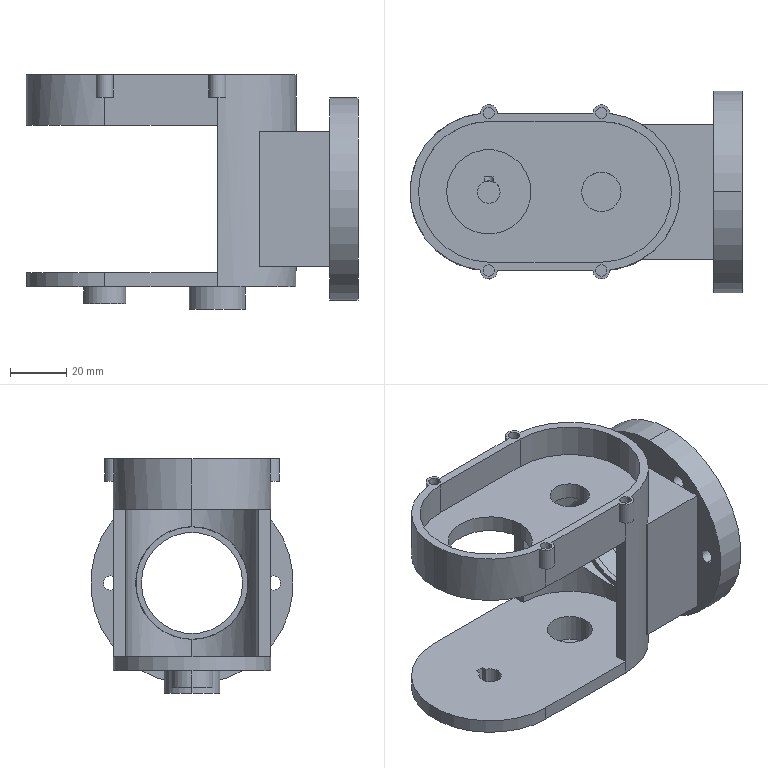Part | SolidWorks | features ICE 17, Cut 1, Extrusion 1 | 1 solid | 101 faces | box 118 x 72 x 83.4 mm | volume 115951 mm3 | cylinder 58 | plane 43 | commonest cylinder face diameters 5 x12 4 x8 6 x6 40 x4 56 x4 50 x3